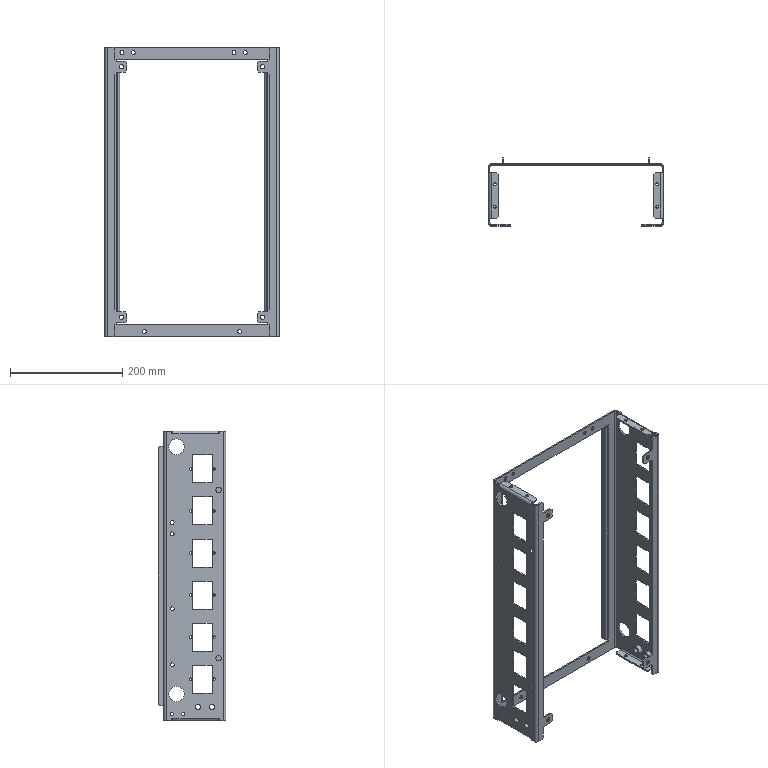Part | STEP file | 64604911 | 1 solid | 370 faces | box 312 x 121 x 517 mm | volume 386207 mm3 | plane 214 | cylinder 156 | commonest cylinder face diameters 4.5 x48 7 x30 5.4 x24 10 x20 5 x8 8 x8